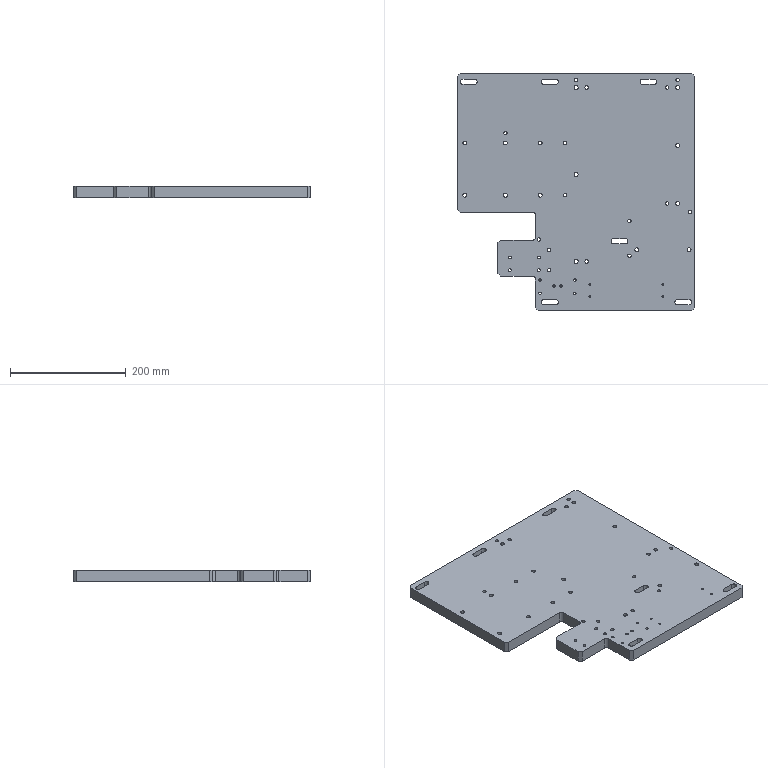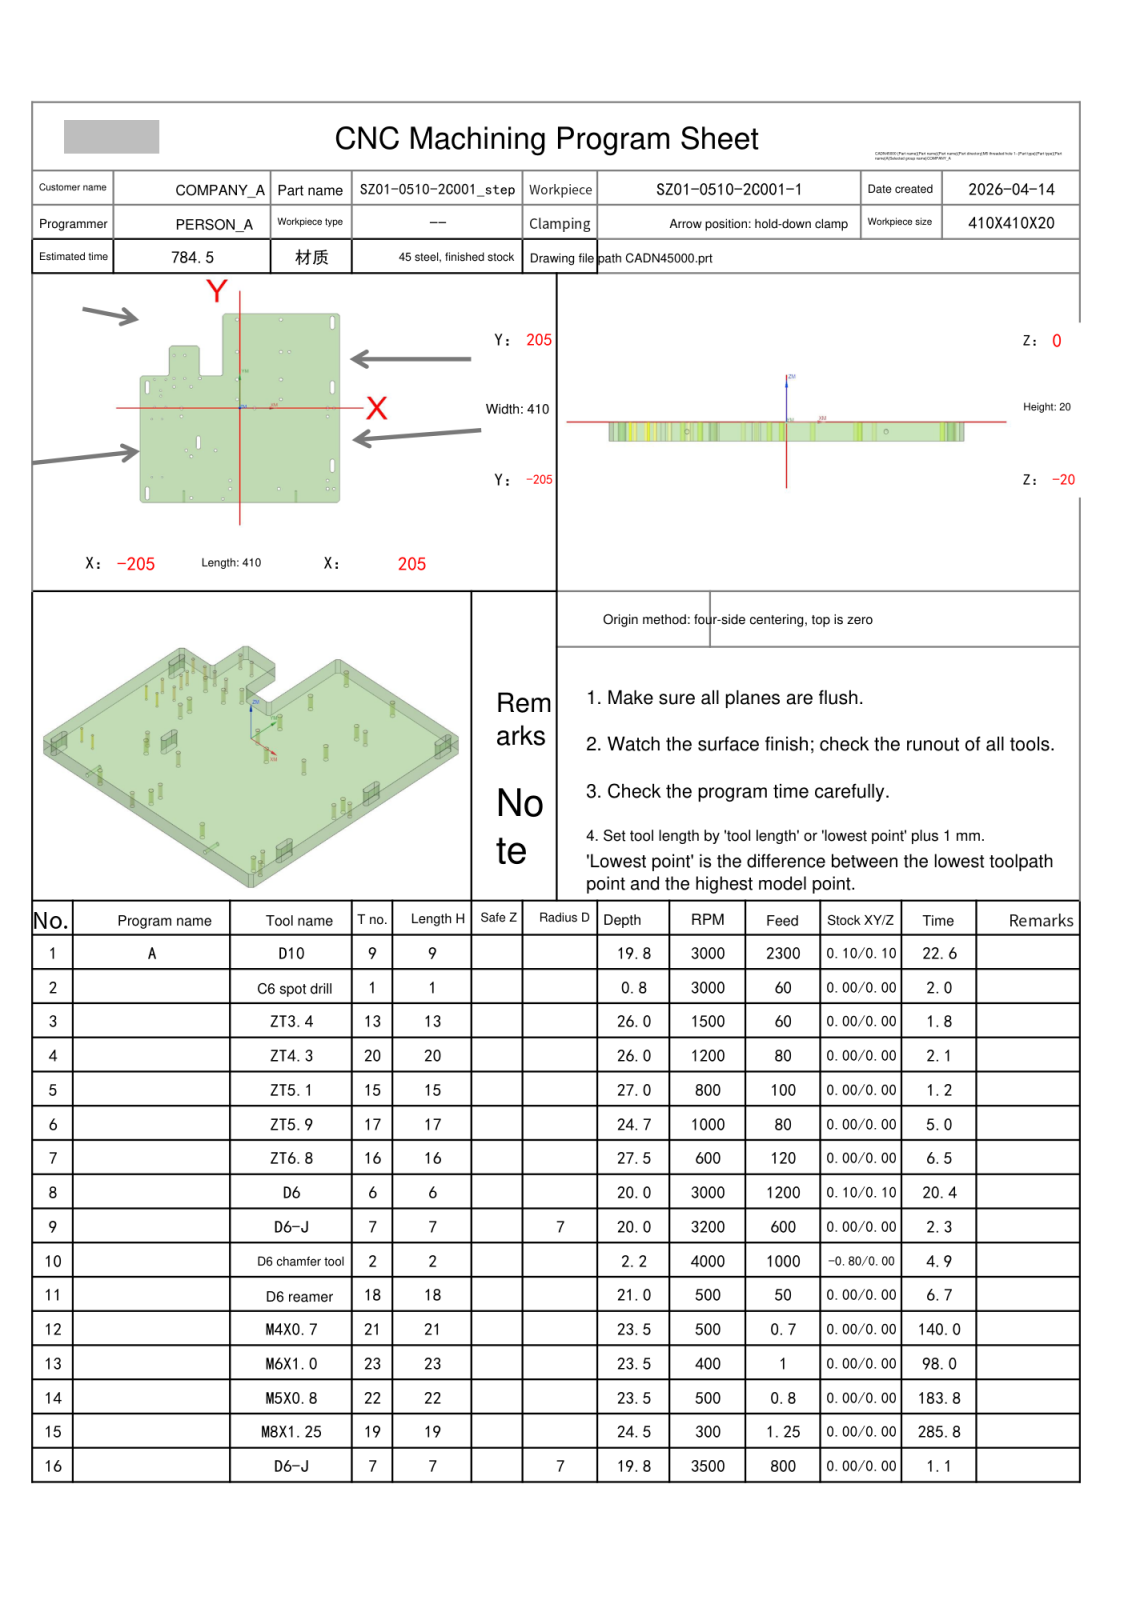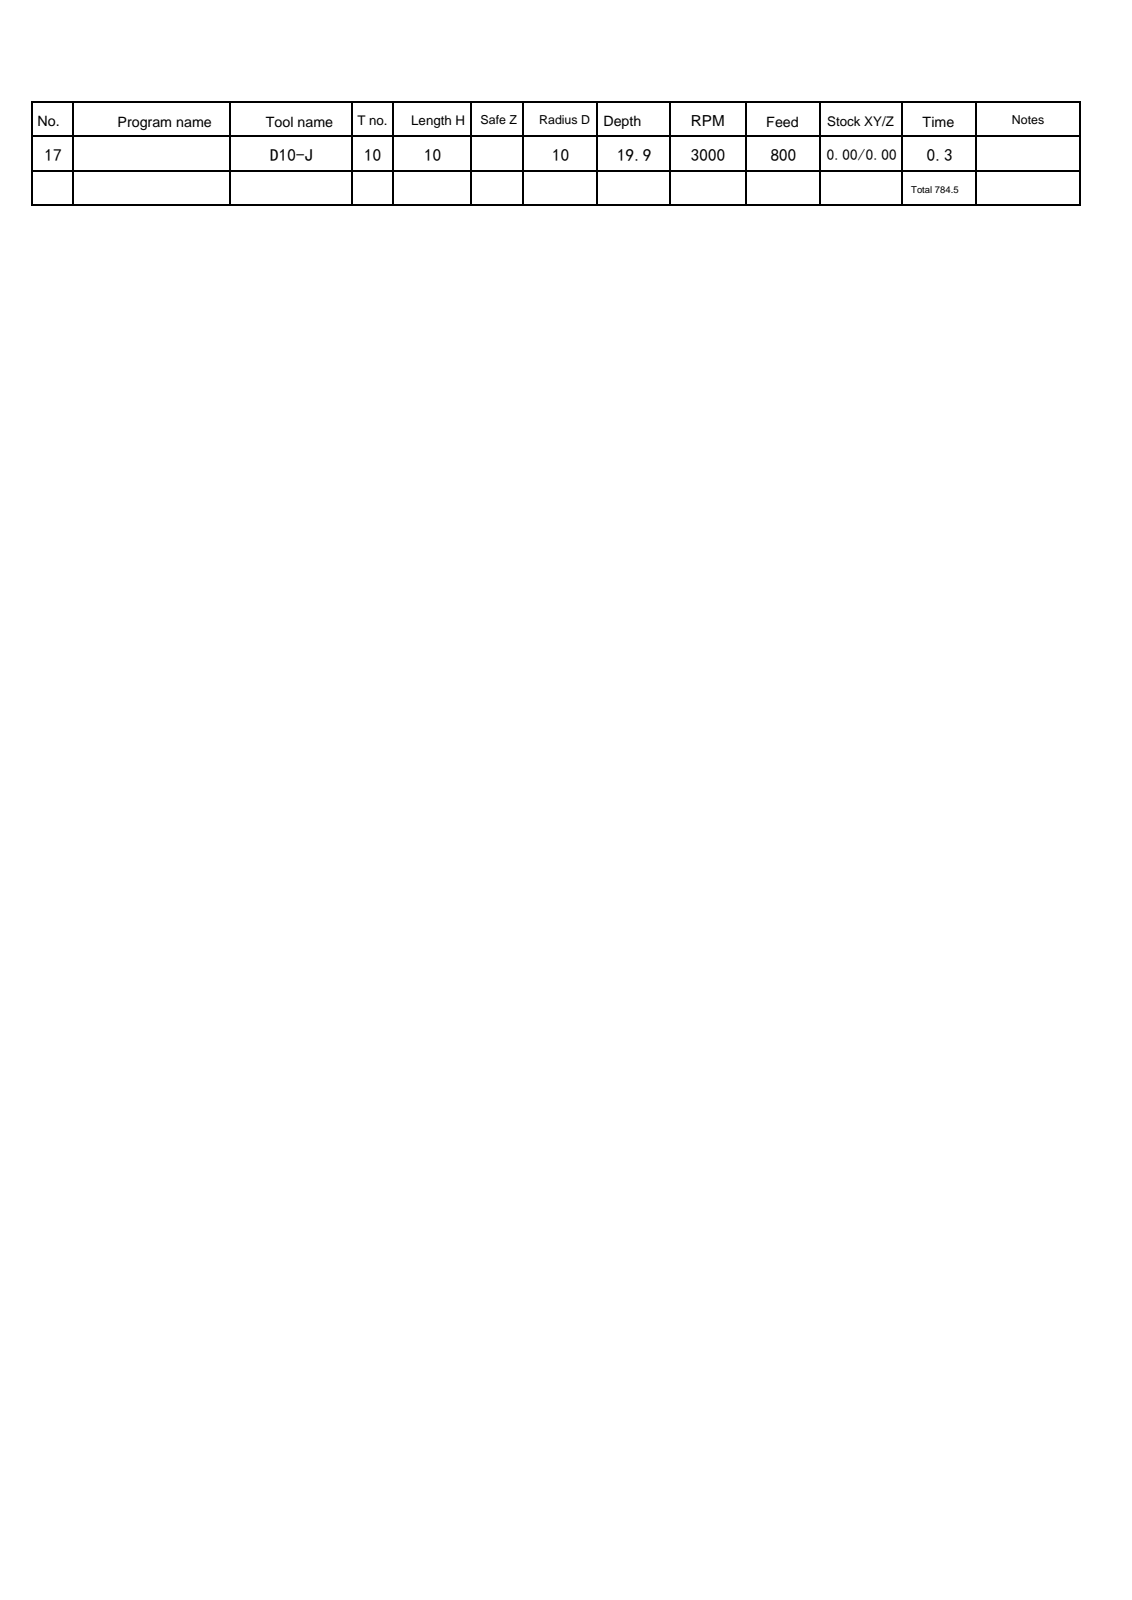NC program | NX | posted by the shop | part box 410 x 410 x 20 mm
Lines 3294 to 4153 of 7905:
N8 T06 M06
(D6  D=6. R=0. H=06 ce=0.10 di=0.10)
G00 G90 G54 X191.4 Y185. M03 S3000
G43 H06 Z50.
M08
Z.5
G01 Y195. Z.449 F1200.
G03 X190. Y196.4 Z.438 I-1.4 J0.0
X188.6 Y195. Z.426 I0.0 J-1.4
G01 Y175. Z.324
G03 X190. Y173.6 Z.313 I1.4 J0.0
X191.4 Y175. Z.301 I0.0 J1.4
G01 Y195. Z.199
G03 X190. Y196.4 Z.188 I-1.4 J0.0
X188.6 Y195. Z.176 I0.0 J-1.4
G01 Y175. Z.074
G03 X190. Y173.6 Z.063 I1.4 J0.0
X191.4 Y175. Z.051 I0.0 J1.4
G01 Y195. Z-.051
G03 X190. Y196.4 Z-.063 I-1.4 J0.0
X188.6 Y195. Z-.074 I0.0 J-1.4
G01 Y175. Z-.176
G03 X190. Y173.6 Z-.188 I1.4 J0.0
X191.4 Y175. Z-.199 I0.0 J1.4
G01 Y195. Z-.301
G03 X190. Y196.4 Z-.313 I-1.4 J0.0
X188.6 Y195. Z-.324 I0.0 J-1.4
G01 Y175. Z-.426
G03 X190. Y173.6 Z-.438 I1.4 J0.0
X191.4 Y175. Z-.449 I0.0 J1.4
G01 Y195. Z-.551
G03 X190. Y196.4 Z-.563 I-1.4 J0.0
X188.6 Y195. Z-.574 I0.0 J-1.4
G01 Y175. Z-.676
G03 X190. Y173.6 Z-.688 I1.4 J0.0
X191.4 Y175. Z-.699 I0.0 J1.4
G01 Y195. Z-.801
G03 X190. Y196.4 Z-.813 I-1.4 J0.0
X188.6 Y195. Z-.824 I0.0 J-1.4
G01 Y175. Z-.926
G03 X190. Y173.6 Z-.938 I1.4 J0.0
X191.4 Y175. Z-.949 I0.0 J1.4
G01 Y195. Z-1.051
G03 X190. Y196.4 Z-1.063 I-1.4 J0.0
X188.6 Y195. Z-1.074 I0.0 J-1.4
G01 Y175. Z-1.176
G03 X190. Y173.6 Z-1.188 I1.4 J0.0
X191.4 Y175. Z-1.199 I0.0 J1.4
G01 Y195. Z-1.301
G03 X190. Y196.4 Z-1.313 I-1.4 J0.0
X188.6 Y195. Z-1.324 I0.0 J-1.4
G01 Y175. Z-1.426
G03 X190. Y173.6 Z-1.438 I1.4 J0.0
X191.4 Y175. Z-1.449 I0.0 J1.4
G01 Y195. Z-1.551
G03 X190. Y196.4 Z-1.563 I-1.4 J0.0
X188.6 Y195. Z-1.574 I0.0 J-1.4
G01 Y175. Z-1.676
G03 X190. Y173.6 Z-1.688 I1.4 J0.0
X191.4 Y175. Z-1.699 I0.0 J1.4
G01 Y195. Z-1.801
G03 X190. Y196.4 Z-1.813 I-1.4 J0.0
X188.6 Y195. Z-1.824 I0.0 J-1.4
G01 Y175. Z-1.926
G03 X190. Y173.6 Z-1.938 I1.4 J0.0
X191.4 Y175. Z-1.949 I0.0 J1.4
G01 Y195. Z-2.051
G03 X190. Y196.4 Z-2.063 I-1.4 J0.0
X188.6 Y195. Z-2.074 I0.0 J-1.4
G01 Y175. Z-2.176
G03 X190. Y173.6 Z-2.188 I1.4 J0.0
X191.4 Y175. Z-2.199 I0.0 J1.4
G01 Y195. Z-2.301
G03 X190. Y196.4 Z-2.313 I-1.4 J0.0
X188.6 Y195. Z-2.324 I0.0 J-1.4
G01 Y175. Z-2.426
G03 X190. Y173.6 Z-2.438 I1.4 J0.0
X191.4 Y175. Z-2.449 I0.0 J1.4
G01 Y195. Z-2.551
G03 X190. Y196.4 Z-2.563 I-1.4 J0.0
X188.6 Y195. Z-2.574 I0.0 J-1.4
G01 Y175. Z-2.676
G03 X190. Y173.6 Z-2.688 I1.4 J0.0
X191.4 Y175. Z-2.699 I0.0 J1.4
G01 Y195. Z-2.801
G03 X190. Y196.4 Z-2.813 I-1.4 J0.0
X188.6 Y195. Z-2.824 I0.0 J-1.4
G01 Y175. Z-2.926
G03 X190. Y173.6 Z-2.938 I1.4 J0.0
X191.4 Y175. Z-2.949 I0.0 J1.4
G01 Y195. Z-3.051
G03 X190. Y196.4 Z-3.063 I-1.4 J0.0
X188.6 Y195. Z-3.074 I0.0 J-1.4
G01 Y175. Z-3.176
G03 X190. Y173.6 Z-3.188 I1.4 J0.0
X191.4 Y175. Z-3.199 I0.0 J1.4
G01 Y195. Z-3.301
G03 X190. Y196.4 Z-3.313 I-1.4 J0.0
X188.6 Y195. Z-3.324 I0.0 J-1.4
G01 Y175. Z-3.426
G03 X190. Y173.6 Z-3.438 I1.4 J0.0
X191.4 Y175. Z-3.449 I0.0 J1.4
G01 Y195. Z-3.551
G03 X190. Y196.4 Z-3.563 I-1.4 J0.0
X188.6 Y195. Z-3.574 I0.0 J-1.4
G01 Y175. Z-3.676
G03 X190. Y173.6 Z-3.688 I1.4 J0.0
X191.4 Y175. Z-3.699 I0.0 J1.4
G01 Y195. Z-3.801
G03 X190. Y196.4 Z-3.813 I-1.4 J0.0
X188.6 Y195. Z-3.824 I0.0 J-1.4
G01 Y175. Z-3.926
G03 X190. Y173.6 Z-3.938 I1.4 J0.0
X191.4 Y175. Z-3.949 I0.0 J1.4
G01 Y195. Z-4.051
G03 X190. Y196.4 Z-4.063 I-1.4 J0.0
X188.6 Y195. Z-4.074 I0.0 J-1.4
G01 Y175. Z-4.176
G03 X190. Y173.6 Z-4.188 I1.4 J0.0
X191.4 Y175. Z-4.199 I0.0 J1.4
G01 Y195. Z-4.301
G03 X190. Y196.4 Z-4.313 I-1.4 J0.0
X188.6 Y195. Z-4.324 I0.0 J-1.4
G01 Y175. Z-4.426
G03 X190. Y173.6 Z-4.438 I1.4 J0.0
X191.4 Y175. Z-4.449 I0.0 J1.4
G01 Y195. Z-4.551
G03 X190. Y196.4 Z-4.563 I-1.4 J0.0
X188.6 Y195. Z-4.574 I0.0 J-1.4
G01 Y175. Z-4.676
G03 X190. Y173.6 Z-4.688 I1.4 J0.0
X191.4 Y175. Z-4.699 I0.0 J1.4
G01 Y195. Z-4.801
G03 X190. Y196.4 Z-4.813 I-1.4 J0.0
X188.6 Y195. Z-4.824 I0.0 J-1.4
G01 Y175. Z-4.926
G03 X190. Y173.6 Z-4.938 I1.4 J0.0
X191.4 Y175. Z-4.949 I0.0 J1.4
G01 Y195. Z-5.051
G03 X190. Y196.4 Z-5.063 I-1.4 J0.0
X188.6 Y195. Z-5.074 I0.0 J-1.4
G01 Y175. Z-5.176
G03 X190. Y173.6 Z-5.188 I1.4 J0.0
X191.4 Y175. Z-5.199 I0.0 J1.4
G01 Y195. Z-5.301
G03 X190. Y196.4 Z-5.313 I-1.4 J0.0
X188.6 Y195. Z-5.324 I0.0 J-1.4
G01 Y175. Z-5.426
G03 X190. Y173.6 Z-5.438 I1.4 J0.0
X191.4 Y175. Z-5.449 I0.0 J1.4
G01 Y195. Z-5.551
G03 X190. Y196.4 Z-5.563 I-1.4 J0.0
X188.6 Y195. Z-5.574 I0.0 J-1.4
G01 Y175. Z-5.676
G03 X190. Y173.6 Z-5.688 I1.4 J0.0
X191.4 Y175. Z-5.699 I0.0 J1.4
G01 Y195. Z-5.801
G03 X190. Y196.4 Z-5.813 I-1.4 J0.0
X188.6 Y195. Z-5.824 I0.0 J-1.4
G01 Y175. Z-5.926
G03 X190. Y173.6 Z-5.938 I1.4 J0.0
X191.4 Y175. Z-5.949 I0.0 J1.4
G01 Y195. Z-6.051
G03 X190. Y196.4 Z-6.063 I-1.4 J0.0
X188.6 Y195. Z-6.074 I0.0 J-1.4
G01 Y175. Z-6.176
G03 X190. Y173.6 Z-6.188 I1.4 J0.0
X191.4 Y175. Z-6.199 I0.0 J1.4
G01 Y195. Z-6.301
G03 X190. Y196.4 Z-6.313 I-1.4 J0.0
X188.6 Y195. Z-6.324 I0.0 J-1.4
G01 Y175. Z-6.426
G03 X190. Y173.6 Z-6.438 I1.4 J0.0
X191.4 Y175. Z-6.449 I0.0 J1.4
G01 Y195. Z-6.551
G03 X190. Y196.4 Z-6.563 I-1.4 J0.0
X188.6 Y195. Z-6.574 I0.0 J-1.4
G01 Y175. Z-6.676
G03 X190. Y173.6 Z-6.688 I1.4 J0.0
X191.4 Y175. Z-6.699 I0.0 J1.4
G01 Y195. Z-6.801
G03 X190. Y196.4 Z-6.813 I-1.4 J0.0
X188.6 Y195. Z-6.824 I0.0 J-1.4
G01 Y175. Z-6.926
G03 X190. Y173.6 Z-6.938 I1.4 J0.0
X191.4 Y175. Z-6.949 I0.0 J1.4
G01 Y195. Z-7.051
G03 X190. Y196.4 Z-7.063 I-1.4 J0.0
X188.6 Y195. Z-7.074 I0.0 J-1.4
G01 Y175. Z-7.176
G03 X190. Y173.6 Z-7.188 I1.4 J0.0
X191.4 Y175. Z-7.199 I0.0 J1.4
G01 Y195. Z-7.301
G03 X190. Y196.4 Z-7.313 I-1.4 J0.0
X188.6 Y195. Z-7.324 I0.0 J-1.4
G01 Y175. Z-7.426
G03 X190. Y173.6 Z-7.438 I1.4 J0.0
X191.4 Y175. Z-7.449 I0.0 J1.4
G01 Y195. Z-7.551
G03 X190. Y196.4 Z-7.563 I-1.4 J0.0
X188.6 Y195. Z-7.574 I0.0 J-1.4
G01 Y175. Z-7.676
G03 X190. Y173.6 Z-7.688 I1.4 J0.0
X191.4 Y175. Z-7.699 I0.0 J1.4
G01 Y195. Z-7.801
G03 X190. Y196.4 Z-7.813 I-1.4 J0.0
X188.6 Y195. Z-7.824 I0.0 J-1.4
G01 Y175. Z-7.926
G03 X190. Y173.6 Z-7.938 I1.4 J0.0
X191.4 Y175. Z-7.949 I0.0 J1.4
G01 Y195. Z-8.051
G03 X190. Y196.4 Z-8.063 I-1.4 J0.0
X188.6 Y195. Z-8.074 I0.0 J-1.4
G01 Y175. Z-8.176
G03 X190. Y173.6 Z-8.188 I1.4 J0.0
X191.4 Y175. Z-8.199 I0.0 J1.4
G01 Y195. Z-8.301
G03 X190. Y196.4 Z-8.313 I-1.4 J0.0
X188.6 Y195. Z-8.324 I0.0 J-1.4
G01 Y175. Z-8.426
G03 X190. Y173.6 Z-8.438 I1.4 J0.0
X191.4 Y175. Z-8.449 I0.0 J1.4
G01 Y195. Z-8.551
G03 X190. Y196.4 Z-8.563 I-1.4 J0.0
X188.6 Y195. Z-8.574 I0.0 J-1.4
G01 Y175. Z-8.676
G03 X190. Y173.6 Z-8.688 I1.4 J0.0
X191.4 Y175. Z-8.699 I0.0 J1.4
G01 Y195. Z-8.801
G03 X190. Y196.4 Z-8.813 I-1.4 J0.0
X188.6 Y195. Z-8.824 I0.0 J-1.4
G01 Y175. Z-8.926
G03 X190. Y173.6 Z-8.938 I1.4 J0.0
X191.4 Y175. Z-8.949 I0.0 J1.4
G01 Y195. Z-9.051
G03 X190. Y196.4 Z-9.063 I-1.4 J0.0
X188.6 Y195. Z-9.074 I0.0 J-1.4
G01 Y175. Z-9.176
G03 X190. Y173.6 Z-9.188 I1.4 J0.0
X191.4 Y175. Z-9.199 I0.0 J1.4
G01 Y195. Z-9.301
G03 X190. Y196.4 Z-9.313 I-1.4 J0.0
X188.6 Y195. Z-9.324 I0.0 J-1.4
G01 Y175. Z-9.426
G03 X190. Y173.6 Z-9.438 I1.4 J0.0
X191.4 Y175. Z-9.449 I0.0 J1.4
G01 Y195. Z-9.551
G03 X190. Y196.4 Z-9.563 I-1.4 J0.0
X188.6 Y195. Z-9.574 I0.0 J-1.4
G01 Y175. Z-9.676
G03 X190. Y173.6 Z-9.688 I1.4 J0.0
X191.4 Y175. Z-9.699 I0.0 J1.4
G01 Y195. Z-9.801
G03 X190. Y196.4 Z-9.813 I-1.4 J0.0
X188.6 Y195. Z-9.824 I0.0 J-1.4
G01 Y175. Z-9.926
G03 X190. Y173.6 Z-9.938 I1.4 J0.0
X191.4 Y175. Z-9.949 I0.0 J1.4
G01 Y195. Z-10.051
G03 X190. Y196.4 Z-10.063 I-1.4 J0.0
X188.6 Y195. Z-10.074 I0.0 J-1.4
G01 Y175. Z-10.176
G03 X190. Y173.6 Z-10.188 I1.4 J0.0
X191.4 Y175. Z-10.199 I0.0 J1.4
G01 Y195. Z-10.301
G03 X190. Y196.4 Z-10.313 I-1.4 J0.0
X188.6 Y195. Z-10.324 I0.0 J-1.4
G01 Y175. Z-10.426
G03 X190. Y173.6 Z-10.438 I1.4 J0.0
X191.4 Y175. Z-10.449 I0.0 J1.4
G01 Y195. Z-10.551
G03 X190. Y196.4 Z-10.563 I-1.4 J0.0
X188.6 Y195. Z-10.574 I0.0 J-1.4
G01 Y175. Z-10.676
G03 X190. Y173.6 Z-10.688 I1.4 J0.0
X191.4 Y175. Z-10.699 I0.0 J1.4
G01 Y195. Z-10.801
G03 X190. Y196.4 Z-10.813 I-1.4 J0.0
X188.6 Y195. Z-10.824 I0.0 J-1.4
G01 Y175. Z-10.926
G03 X190. Y173.6 Z-10.938 I1.4 J0.0
X191.4 Y175. Z-10.949 I0.0 J1.4
G01 Y195. Z-11.051
G03 X190. Y196.4 Z-11.063 I-1.4 J0.0
X188.6 Y195. Z-11.074 I0.0 J-1.4
G01 Y175. Z-11.176
G03 X190. Y173.6 Z-11.188 I1.4 J0.0
X191.4 Y175. Z-11.199 I0.0 J1.4
G01 Y195. Z-11.301
G03 X190. Y196.4 Z-11.313 I-1.4 J0.0
X188.6 Y195. Z-11.324 I0.0 J-1.4
G01 Y175. Z-11.426
G03 X190. Y173.6 Z-11.438 I1.4 J0.0
X191.4 Y175. Z-11.449 I0.0 J1.4
G01 Y195. Z-11.551
G03 X190. Y196.4 Z-11.563 I-1.4 J0.0
X188.6 Y195. Z-11.574 I0.0 J-1.4
G01 Y175. Z-11.676
G03 X190. Y173.6 Z-11.688 I1.4 J0.0
X191.4 Y175. Z-11.699 I0.0 J1.4
G01 Y195. Z-11.801
G03 X190. Y196.4 Z-11.813 I-1.4 J0.0
X188.6 Y195. Z-11.824 I0.0 J-1.4
G01 Y175. Z-11.926
G03 X190. Y173.6 Z-11.938 I1.4 J0.0
X191.4 Y175. Z-11.949 I0.0 J1.4
G01 Y195. Z-12.051
G03 X190. Y196.4 Z-12.063 I-1.4 J0.0
X188.6 Y195. Z-12.074 I0.0 J-1.4
G01 Y175. Z-12.176
G03 X190. Y173.6 Z-12.188 I1.4 J0.0
X191.4 Y175. Z-12.199 I0.0 J1.4
G01 Y195. Z-12.301
G03 X190. Y196.4 Z-12.313 I-1.4 J0.0
X188.6 Y195. Z-12.324 I0.0 J-1.4
G01 Y175. Z-12.426
G03 X190. Y173.6 Z-12.438 I1.4 J0.0
X191.4 Y175. Z-12.449 I0.0 J1.4
G01 Y195. Z-12.551
G03 X190. Y196.4 Z-12.563 I-1.4 J0.0
X188.6 Y195. Z-12.574 I0.0 J-1.4
G01 Y175. Z-12.676
G03 X190. Y173.6 Z-12.688 I1.4 J0.0
X191.4 Y175. Z-12.699 I0.0 J1.4
G01 Y195. Z-12.801
G03 X190. Y196.4 Z-12.813 I-1.4 J0.0
X188.6 Y195. Z-12.824 I0.0 J-1.4
G01 Y175. Z-12.926
G03 X190. Y173.6 Z-12.938 I1.4 J0.0
X191.4 Y175. Z-12.949 I0.0 J1.4
G01 Y195. Z-13.051
G03 X190. Y196.4 Z-13.063 I-1.4 J0.0
X188.6 Y195. Z-13.074 I0.0 J-1.4
G01 Y175. Z-13.176
G03 X190. Y173.6 Z-13.188 I1.4 J0.0
X191.4 Y175. Z-13.199 I0.0 J1.4
G01 Y195. Z-13.301
G03 X190. Y196.4 Z-13.313 I-1.4 J0.0
X188.6 Y195. Z-13.324 I0.0 J-1.4
G01 Y175. Z-13.426
G03 X190. Y173.6 Z-13.438 I1.4 J0.0
X191.4 Y175. Z-13.449 I0.0 J1.4
G01 Y195. Z-13.551
G03 X190. Y196.4 Z-13.563 I-1.4 J0.0
X188.6 Y195. Z-13.574 I0.0 J-1.4
G01 Y175. Z-13.676
G03 X190. Y173.6 Z-13.688 I1.4 J0.0
X191.4 Y175. Z-13.699 I0.0 J1.4
G01 Y195. Z-13.801
G03 X190. Y196.4 Z-13.813 I-1.4 J0.0
X188.6 Y195. Z-13.824 I0.0 J-1.4
G01 Y175. Z-13.926
G03 X190. Y173.6 Z-13.938 I1.4 J0.0
X191.4 Y175. Z-13.949 I0.0 J1.4
G01 Y195. Z-14.051
G03 X190. Y196.4 Z-14.063 I-1.4 J0.0
X188.6 Y195. Z-14.074 I0.0 J-1.4
G01 Y175. Z-14.176
G03 X190. Y173.6 Z-14.188 I1.4 J0.0
X191.4 Y175. Z-14.199 I0.0 J1.4
G01 Y195. Z-14.301
G03 X190. Y196.4 Z-14.313 I-1.4 J0.0
X188.6 Y195. Z-14.324 I0.0 J-1.4
G01 Y175. Z-14.426
G03 X190. Y173.6 Z-14.438 I1.4 J0.0
X191.4 Y175. Z-14.449 I0.0 J1.4
G01 Y195. Z-14.551
G03 X190. Y196.4 Z-14.563 I-1.4 J0.0
X188.6 Y195. Z-14.574 I0.0 J-1.4
G01 Y175. Z-14.676
G03 X190. Y173.6 Z-14.688 I1.4 J0.0
X191.4 Y175. Z-14.699 I0.0 J1.4
G01 Y195. Z-14.801
G03 X190. Y196.4 Z-14.813 I-1.4 J0.0
X188.6 Y195. Z-14.824 I0.0 J-1.4
G01 Y175. Z-14.926
G03 X190. Y173.6 Z-14.938 I1.4 J0.0
X191.4 Y175. Z-14.949 I0.0 J1.4
G01 Y195. Z-15.051
G03 X190. Y196.4 Z-15.063 I-1.4 J0.0
X188.6 Y195. Z-15.074 I0.0 J-1.4
G01 Y175. Z-15.176
G03 X190. Y173.6 Z-15.188 I1.4 J0.0
X191.4 Y175. Z-15.199 I0.0 J1.4
G01 Y195. Z-15.301
G03 X190. Y196.4 Z-15.313 I-1.4 J0.0
X188.6 Y195. Z-15.324 I0.0 J-1.4
G01 Y175. Z-15.426
G03 X190. Y173.6 Z-15.438 I1.4 J0.0
X191.4 Y175. Z-15.449 I0.0 J1.4
G01 Y195. Z-15.551
G03 X190. Y196.4 Z-15.563 I-1.4 J0.0
X188.6 Y195. Z-15.574 I0.0 J-1.4
G01 Y175. Z-15.676
G03 X190. Y173.6 Z-15.688 I1.4 J0.0
X191.4 Y175. Z-15.699 I0.0 J1.4
G01 Y195. Z-15.801
G03 X190. Y196.4 Z-15.813 I-1.4 J0.0
X188.6 Y195. Z-15.824 I0.0 J-1.4
G01 Y175. Z-15.926
G03 X190. Y173.6 Z-15.938 I1.4 J0.0
X191.4 Y175. Z-15.949 I0.0 J1.4
G01 Y195. Z-16.051
G03 X190. Y196.4 Z-16.063 I-1.4 J0.0
X188.6 Y195. Z-16.074 I0.0 J-1.4
G01 Y175. Z-16.176
G03 X190. Y173.6 Z-16.188 I1.4 J0.0
X191.4 Y175. Z-16.199 I0.0 J1.4
G01 Y195. Z-16.301
G03 X190. Y196.4 Z-16.313 I-1.4 J0.0
X188.6 Y195. Z-16.324 I0.0 J-1.4
G01 Y175. Z-16.426
G03 X190. Y173.6 Z-16.438 I1.4 J0.0
X191.4 Y175. Z-16.449 I0.0 J1.4
G01 Y195. Z-16.551
G03 X190. Y196.4 Z-16.563 I-1.4 J0.0
X188.6 Y195. Z-16.574 I0.0 J-1.4
G01 Y175. Z-16.676
G03 X190. Y173.6 Z-16.688 I1.4 J0.0
X191.4 Y175. Z-16.699 I0.0 J1.4
G01 Y195. Z-16.801
G03 X190. Y196.4 Z-16.813 I-1.4 J0.0
X188.6 Y195. Z-16.824 I0.0 J-1.4
G01 Y175. Z-16.926
G03 X190. Y173.6 Z-16.938 I1.4 J0.0
X191.4 Y175. Z-16.949 I0.0 J1.4
G01 Y195. Z-17.051
G03 X190. Y196.4 Z-17.063 I-1.4 J0.0
X188.6 Y195. Z-17.074 I0.0 J-1.4
G01 Y175. Z-17.176
G03 X190. Y173.6 Z-17.188 I1.4 J0.0
X191.4 Y175. Z-17.199 I0.0 J1.4
G01 Y195. Z-17.301
G03 X190. Y196.4 Z-17.313 I-1.4 J0.0
X188.6 Y195. Z-17.324 I0.0 J-1.4
G01 Y175. Z-17.426
G03 X190. Y173.6 Z-17.438 I1.4 J0.0
X191.4 Y175. Z-17.449 I0.0 J1.4
G01 Y195. Z-17.551
G03 X190. Y196.4 Z-17.563 I-1.4 J0.0
X188.6 Y195. Z-17.574 I0.0 J-1.4
G01 Y175. Z-17.676
G03 X190. Y173.6 Z-17.688 I1.4 J0.0
X191.4 Y175. Z-17.699 I0.0 J1.4
G01 Y195. Z-17.801
G03 X190. Y196.4 Z-17.813 I-1.4 J0.0
X188.6 Y195. Z-17.824 I0.0 J-1.4
G01 Y175. Z-17.926
G03 X190. Y173.6 Z-17.938 I1.4 J0.0
X191.4 Y175. Z-17.949 I0.0 J1.4
G01 Y195. Z-18.051
G03 X190. Y196.4 Z-18.063 I-1.4 J0.0
X188.6 Y195. Z-18.074 I0.0 J-1.4
G01 Y175. Z-18.176
G03 X190. Y173.6 Z-18.188 I1.4 J0.0
X191.4 Y175. Z-18.199 I0.0 J1.4
G01 Y195. Z-18.301
G03 X190. Y196.4 Z-18.313 I-1.4 J0.0
X188.6 Y195. Z-18.324 I0.0 J-1.4
G01 Y175. Z-18.426
G03 X190. Y173.6 Z-18.438 I1.4 J0.0
X191.4 Y175. Z-18.449 I0.0 J1.4
G01 Y195. Z-18.551
G03 X190. Y196.4 Z-18.563 I-1.4 J0.0
X188.6 Y195. Z-18.574 I0.0 J-1.4
G01 Y175. Z-18.676
G03 X190. Y173.6 Z-18.688 I1.4 J0.0
X191.4 Y175. Z-18.699 I0.0 J1.4
G01 Y195. Z-18.801
G03 X190. Y196.4 Z-18.813 I-1.4 J0.0
X188.6 Y195. Z-18.824 I0.0 J-1.4
G01 Y175. Z-18.926
G03 X190. Y173.6 Z-18.938 I1.4 J0.0
X191.4 Y175. Z-18.949 I0.0 J1.4
G01 Y195. Z-19.051
G03 X190. Y196.4 Z-19.063 I-1.4 J0.0
X188.6 Y195. Z-19.074 I0.0 J-1.4
G01 Y175. Z-19.176
G03 X190. Y173.6 Z-19.188 I1.4 J0.0
X191.4 Y175. Z-19.199 I0.0 J1.4
G01 Y195. Z-19.301
G03 X190. Y196.4 Z-19.313 I-1.4 J0.0
X188.6 Y195. Z-19.324 I0.0 J-1.4
G01 Y175. Z-19.426
G03 X190. Y173.6 Z-19.438 I1.4 J0.0
X191.4 Y175. Z-19.449 I0.0 J1.4
G01 Y195. Z-19.551
G03 X190. Y196.4 Z-19.563 I-1.4 J0.0
X188.6 Y195. Z-19.574 I0.0 J-1.4
G01 Y175. Z-19.676
G03 X190. Y173.6 Z-19.688 I1.4 J0.0
X191.4 Y175. Z-19.699 I0.0 J1.4
G01 Y195. Z-19.801
G03 X190. Y196.4 Z-19.813 I-1.4 J0.0
X188.6 Y195. Z-19.824 I0.0 J-1.4
G01 Y175. Z-19.926
G03 X190. Y173.6 Z-19.938 I1.4 J0.0
X191.4 Y175. Z-19.949 I0.0 J1.4
G01 Y185. Z-20.
Y195.
G03 X190. Y196.4 I-1.4 J0.0
X188.6 Y195. I0.0 J-1.4
G01 Y175.
G03 X190. Y173.6 I1.4 J0.0
X191.4 Y175. I0.0 J1.4
G01 Y185.
Y185.5
Z-19.
G00 Z50.
Y45.
Z.5
G01 Y55. Z.449
G03 X190. Y56.4 Z.438 I-1.4 J0.0
X188.6 Y55. Z.426 I0.0 J-1.4
G01 Y35. Z.324
G03 X190. Y33.6 Z.313 I1.4 J0.0
X191.4 Y35. Z.301 I0.0 J1.4
G01 Y55. Z.199
G03 X190. Y56.4 Z.188 I-1.4 J0.0
X188.6 Y55. Z.176 I0.0 J-1.4
G01 Y35. Z.074
G03 X190. Y33.6 Z.063 I1.4 J0.0
X191.4 Y35. Z.051 I0.0 J1.4
G01 Y55. Z-.051
G03 X190. Y56.4 Z-.063 I-1.4 J0.0
X188.6 Y55. Z-.074 I0.0 J-1.4
G01 Y35. Z-.176
G03 X190. Y33.6 Z-.188 I1.4 J0.0
X191.4 Y35. Z-.199 I0.0 J1.4
G01 Y55. Z-.301
G03 X190. Y56.4 Z-.313 I-1.4 J0.0
X188.6 Y55. Z-.324 I0.0 J-1.4
G01 Y35. Z-.426
G03 X190. Y33.6 Z-.438 I1.4 J0.0
X191.4 Y35. Z-.449 I0.0 J1.4
G01 Y55. Z-.551
G03 X190. Y56.4 Z-.563 I-1.4 J0.0
X188.6 Y55. Z-.574 I0.0 J-1.4
G01 Y35. Z-.676
G03 X190. Y33.6 Z-.688 I1.4 J0.0
X191.4 Y35. Z-.699 I0.0 J1.4
G01 Y55. Z-.801
G03 X190. Y56.4 Z-.813 I-1.4 J0.0
X188.6 Y55. Z-.824 I0.0 J-1.4
G01 Y35. Z-.926
G03 X190. Y33.6 Z-.938 I1.4 J0.0
X191.4 Y35. Z-.949 I0.0 J1.4
G01 Y55. Z-1.051
G03 X190. Y56.4 Z-1.063 I-1.4 J0.0
X188.6 Y55. Z-1.074 I0.0 J-1.4
G01 Y35. Z-1.176
G03 X190. Y33.6 Z-1.188 I1.4 J0.0
X191.4 Y35. Z-1.199 I0.0 J1.4
G01 Y55. Z-1.301
G03 X190. Y56.4 Z-1.313 I-1.4 J0.0
X188.6 Y55. Z-1.324 I0.0 J-1.4
G01 Y35. Z-1.426
G03 X190. Y33.6 Z-1.438 I1.4 J0.0
X191.4 Y35. Z-1.449 I0.0 J1.4
G01 Y55. Z-1.551
G03 X190. Y56.4 Z-1.563 I-1.4 J0.0
X188.6 Y55. Z-1.574 I0.0 J-1.4
G01 Y35. Z-1.676
G03 X190. Y33.6 Z-1.688 I1.4 J0.0
X191.4 Y35. Z-1.699 I0.0 J1.4
G01 Y55. Z-1.801
G03 X190. Y56.4 Z-1.813 I-1.4 J0.0
X188.6 Y55. Z-1.824 I0.0 J-1.4
G01 Y35. Z-1.926
G03 X190. Y33.6 Z-1.938 I1.4 J0.0
X191.4 Y35. Z-1.949 I0.0 J1.4
G01 Y55. Z-2.051
G03 X190. Y56.4 Z-2.063 I-1.4 J0.0
X188.6 Y55. Z-2.074 I0.0 J-1.4
G01 Y35. Z-2.176
G03 X190. Y33.6 Z-2.188 I1.4 J0.0
X191.4 Y35. Z-2.199 I0.0 J1.4
G01 Y55. Z-2.301
G03 X190. Y56.4 Z-2.313 I-1.4 J0.0
X188.6 Y55. Z-2.324 I0.0 J-1.4
G01 Y35. Z-2.426
G03 X190. Y33.6 Z-2.438 I1.4 J0.0
X191.4 Y35. Z-2.449 I0.0 J1.4
G01 Y55. Z-2.551
G03 X190. Y56.4 Z-2.563 I-1.4 J0.0
X188.6 Y55. Z-2.574 I0.0 J-1.4
G01 Y35. Z-2.676
G03 X190. Y33.6 Z-2.688 I1.4 J0.0
X191.4 Y35. Z-2.699 I0.0 J1.4
G01 Y55. Z-2.801
G03 X190. Y56.4 Z-2.813 I-1.4 J0.0
X188.6 Y55. Z-2.824 I0.0 J-1.4
G01 Y35. Z-2.926
G03 X190. Y33.6 Z-2.938 I1.4 J0.0
X191.4 Y35. Z-2.949 I0.0 J1.4
G01 Y55. Z-3.051
G03 X190. Y56.4 Z-3.063 I-1.4 J0.0
X188.6 Y55. Z-3.074 I0.0 J-1.4
G01 Y35. Z-3.176
G03 X190. Y33.6 Z-3.188 I1.4 J0.0
X191.4 Y35. Z-3.199 I0.0 J1.4
G01 Y55. Z-3.301
G03 X190. Y56.4 Z-3.313 I-1.4 J0.0
X188.6 Y55. Z-3.324 I0.0 J-1.4
G01 Y35. Z-3.426
G03 X190. Y33.6 Z-3.438 I1.4 J0.0
X191.4 Y35. Z-3.449 I0.0 J1.4
G01 Y55. Z-3.551
G03 X190. Y56.4 Z-3.563 I-1.4 J0.0
X188.6 Y55. Z-3.574 I0.0 J-1.4
G01 Y35. Z-3.676
G03 X190. Y33.6 Z-3.688 I1.4 J0.0
X191.4 Y35. Z-3.699 I0.0 J1.4
G01 Y55. Z-3.801
G03 X190. Y56.4 Z-3.813 I-1.4 J0.0
X188.6 Y55. Z-3.824 I0.0 J-1.4
G01 Y35. Z-3.926
G03 X190. Y33.6 Z-3.938 I1.4 J0.0
X191.4 Y35. Z-3.949 I0.0 J1.4
G01 Y55. Z-4.051
G03 X190. Y56.4 Z-4.063 I-1.4 J0.0
X188.6 Y55. Z-4.074 I0.0 J-1.4
G01 Y35. Z-4.176
G03 X190. Y33.6 Z-4.188 I1.4 J0.0
X191.4 Y35. Z-4.199 I0.0 J1.4
G01 Y55. Z-4.301
G03 X190. Y56.4 Z-4.313 I-1.4 J0.0
X188.6 Y55. Z-4.324 I0.0 J-1.4
G01 Y35. Z-4.426
G03 X190. Y33.6 Z-4.438 I1.4 J0.0
X191.4 Y35. Z-4.449 I0.0 J1.4
G01 Y55. Z-4.551
G03 X190. Y56.4 Z-4.563 I-1.4 J0.0
X188.6 Y55. Z-4.574 I0.0 J-1.4
G01 Y35. Z-4.676
G03 X190. Y33.6 Z-4.688 I1.4 J0.0
X191.4 Y35. Z-4.699 I0.0 J1.4
G01 Y55. Z-4.801
G03 X190. Y56.4 Z-4.813 I-1.4 J0.0
X188.6 Y55. Z-4.824 I0.0 J-1.4
G01 Y35. Z-4.926
G03 X190. Y33.6 Z-4.938 I1.4 J0.0
X191.4 Y35. Z-4.949 I0.0 J1.4
G01 Y55. Z-5.051
G03 X190. Y56.4 Z-5.063 I-1.4 J0.0
X188.6 Y55. Z-5.074 I0.0 J-1.4
G01 Y35. Z-5.176
G03 X190. Y33.6 Z-5.188 I1.4 J0.0
X191.4 Y35. Z-5.199 I0.0 J1.4
G01 Y55. Z-5.301
G03 X190. Y56.4 Z-5.313 I-1.4 J0.0
X188.6 Y55. Z-5.324 I0.0 J-1.4
G01 Y35. Z-5.426
G03 X190. Y33.6 Z-5.438 I1.4 J0.0
X191.4 Y35. Z-5.449 I0.0 J1.4
G01 Y55. Z-5.551
G03 X190. Y56.4 Z-5.563 I-1.4 J0.0
X188.6 Y55. Z-5.574 I0.0 J-1.4
G01 Y35. Z-5.676
G03 X190. Y33.6 Z-5.688 I1.4 J0.0
X191.4 Y35. Z-5.699 I0.0 J1.4
G01 Y55. Z-5.801
G03 X190. Y56.4 Z-5.813 I-1.4 J0.0
X188.6 Y55. Z-5.824 I0.0 J-1.4
G01 Y35. Z-5.926
G03 X190. Y33.6 Z-5.938 I1.4 J0.0
X191.4 Y35. Z-5.949 I0.0 J1.4
G01 Y55. Z-6.051
G03 X190. Y56.4 Z-6.063 I-1.4 J0.0
X188.6 Y55. Z-6.074 I0.0 J-1.4
G01 Y35. Z-6.176
G03 X190. Y33.6 Z-6.188 I1.4 J0.0
X191.4 Y35. Z-6.199 I0.0 J1.4
G01 Y55. Z-6.301
G03 X190. Y56.4 Z-6.313 I-1.4 J0.0
X188.6 Y55. Z-6.324 I0.0 J-1.4
G01 Y35. Z-6.426
G03 X190. Y33.6 Z-6.438 I1.4 J0.0
X191.4 Y35. Z-6.449 I0.0 J1.4
G01 Y55. Z-6.551
G03 X190. Y56.4 Z-6.563 I-1.4 J0.0
X188.6 Y55. Z-6.574 I0.0 J-1.4
G01 Y35. Z-6.676
G03 X190. Y33.6 Z-6.688 I1.4 J0.0
X191.4 Y35. Z-6.699 I0.0 J1.4
G01 Y55. Z-6.801
G03 X190. Y56.4 Z-6.813 I-1.4 J0.0
X188.6 Y55. Z-6.824 I0.0 J-1.4
G01 Y35. Z-6.926
G03 X190. Y33.6 Z-6.938 I1.4 J0.0
X191.4 Y35. Z-6.949 I0.0 J1.4
G01 Y55. Z-7.051
G03 X190. Y56.4 Z-7.063 I-1.4 J0.0
X188.6 Y55. Z-7.074 I0.0 J-1.4
G01 Y35. Z-7.176
G03 X190. Y33.6 Z-7.188 I1.4 J0.0
X191.4 Y35. Z-7.199 I0.0 J1.4
G01 Y55. Z-7.301
G03 X190. Y56.4 Z-7.313 I-1.4 J0.0
X188.6 Y55. Z-7.324 I0.0 J-1.4
G01 Y35. Z-7.426
G03 X190. Y33.6 Z-7.438 I1.4 J0.0
X191.4 Y35. Z-7.449 I0.0 J1.4
G01 Y55. Z-7.551
G03 X190. Y56.4 Z-7.563 I-1.4 J0.0
X188.6 Y55. Z-7.574 I0.0 J-1.4
G01 Y35. Z-7.676
G03 X190. Y33.6 Z-7.688 I1.4 J0.0
X191.4 Y35. Z-7.699 I0.0 J1.4
G01 Y55. Z-7.801
G03 X190. Y56.4 Z-7.813 I-1.4 J0.0
X188.6 Y55. Z-7.824 I0.0 J-1.4
G01 Y35. Z-7.926
G03 X190. Y33.6 Z-7.938 I1.4 J0.0
X191.4 Y35. Z-7.949 I0.0 J1.4
G01 Y55. Z-8.051
G03 X190. Y56.4 Z-8.063 I-1.4 J0.0
X188.6 Y55. Z-8.074 I0.0 J-1.4
G01 Y35. Z-8.176
G03 X190. Y33.6 Z-8.188 I1.4 J0.0
X191.4 Y35. Z-8.199 I0.0 J1.4
G01 Y55. Z-8.301
G03 X190. Y56.4 Z-8.313 I-1.4 J0.0
X188.6 Y55. Z-8.324 I0.0 J-1.4
G01 Y35. Z-8.426
G03 X190. Y33.6 Z-8.438 I1.4 J0.0
X191.4 Y35. Z-8.449 I0.0 J1.4
G01 Y55. Z-8.551
G03 X190. Y56.4 Z-8.563 I-1.4 J0.0
X188.6 Y55. Z-8.574 I0.0 J-1.4
G01 Y35. Z-8.676
G03 X190. Y33.6 Z-8.688 I1.4 J0.0
X191.4 Y35. Z-8.699 I0.0 J1.4
G01 Y55. Z-8.801
G03 X190. Y56.4 Z-8.813 I-1.4 J0.0
X188.6 Y55. Z-8.824 I0.0 J-1.4
G01 Y35. Z-8.926
G03 X190. Y33.6 Z-8.938 I1.4 J0.0
X191.4 Y35. Z-8.949 I0.0 J1.4
G01 Y55. Z-9.051
G03 X190. Y56.4 Z-9.063 I-1.4 J0.0
X188.6 Y55. Z-9.074 I0.0 J-1.4
G01 Y35. Z-9.176
G03 X190. Y33.6 Z-9.188 I1.4 J0.0
X191.4 Y35. Z-9.199 I0.0 J1.4
G01 Y55. Z-9.301
G03 X190. Y56.4 Z-9.313 I-1.4 J0.0
X188.6 Y55. Z-9.324 I0.0 J-1.4
G01 Y35. Z-9.426
G03 X190. Y33.6 Z-9.438 I1.4 J0.0
X191.4 Y35. Z-9.449 I0.0 J1.4
G01 Y55. Z-9.551
G03 X190. Y56.4 Z-9.563 I-1.4 J0.0
X188.6 Y55. Z-9.574 I0.0 J-1.4
G01 Y35. Z-9.676
G03 X190. Y33.6 Z-9.688 I1.4 J0.0
X191.4 Y35. Z-9.699 I0.0 J1.4
G01 Y55. Z-9.801
G03 X190. Y56.4 Z-9.813 I-1.4 J0.0
X188.6 Y55. Z-9.824 I0.0 J-1.4
G01 Y35. Z-9.926
G03 X190. Y33.6 Z-9.938 I1.4 J0.0
X191.4 Y35. Z-9.949 I0.0 J1.4
G01 Y55. Z-10.051
G03 X190. Y56.4 Z-10.063 I-1.4 J0.0
X188.6 Y55. Z-10.074 I0.0 J-1.4
G01 Y35. Z-10.176
G03 X190. Y33.6 Z-10.188 I1.4 J0.0
X191.4 Y35. Z-10.199 I0.0 J1.4
G01 Y55. Z-10.301
G03 X190. Y56.4 Z-10.313 I-1.4 J0.0
X188.6 Y55. Z-10.324 I0.0 J-1.4
G01 Y35. Z-10.426
G03 X190. Y33.6 Z-10.438 I1.4 J0.0
X191.4 Y35. Z-10.449 I0.0 J1.4
G01 Y55. Z-10.551
G03 X190. Y56.4 Z-10.563 I-1.4 J0.0
X188.6 Y55. Z-10.574 I0.0 J-1.4
G01 Y35. Z-10.676
G03 X190. Y33.6 Z-10.688 I1.4 J0.0
X191.4 Y35. Z-10.699 I0.0 J1.4
G01 Y55. Z-10.801
G03 X190. Y56.4 Z-10.813 I-1.4 J0.0
X188.6 Y55. Z-10.824 I0.0 J-1.4
G01 Y35. Z-10.926
G03 X190. Y33.6 Z-10.938 I1.4 J0.0
X191.4 Y35. Z-10.949 I0.0 J1.4
G01 Y55. Z-11.051
G03 X190. Y56.4 Z-11.063 I-1.4 J0.0
X188.6 Y55. Z-11.074 I0.0 J-1.4
G01 Y35. Z-11.176
G03 X190. Y33.6 Z-11.188 I1.4 J0.0
X191.4 Y35. Z-11.199 I0.0 J1.4
G01 Y55. Z-11.301
G03 X190. Y56.4 Z-11.313 I-1.4 J0.0
X188.6 Y55. Z-11.324 I0.0 J-1.4
G01 Y35. Z-11.426
G03 X190. Y33.6 Z-11.438 I1.4 J0.0
X191.4 Y35. Z-11.449 I0.0 J1.4
G01 Y55. Z-11.551
G03 X190. Y56.4 Z-11.563 I-1.4 J0.0
X188.6 Y55. Z-11.574 I0.0 J-1.4
G01 Y35. Z-11.676
G03 X190. Y33.6 Z-11.688 I1.4 J0.0
X191.4 Y35. Z-11.699 I0.0 J1.4
G01 Y55. Z-11.801
G03 X190. Y56.4 Z-11.813 I-1.4 J0.0
X188.6 Y55. Z-11.824 I0.0 J-1.4
G01 Y35. Z-11.926
G03 X190. Y33.6 Z-11.938 I1.4 J0.0
X191.4 Y35. Z-11.949 I0.0 J1.4
G01 Y55. Z-12.051
G03 X190. Y56.4 Z-12.063 I-1.4 J0.0
X188.6 Y55. Z-12.074 I0.0 J-1.4
G01 Y35. Z-12.176
G03 X190. Y33.6 Z-12.188 I1.4 J0.0
X191.4 Y35. Z-12.199 I0.0 J1.4
G01 Y55. Z-12.301
G03 X190. Y56.4 Z-12.313 I-1.4 J0.0
X188.6 Y55. Z-12.324 I0.0 J-1.4
G01 Y35. Z-12.426
G03 X190. Y33.6 Z-12.438 I1.4 J0.0
X191.4 Y35. Z-12.449 I0.0 J1.4
G01 Y55. Z-12.551
G03 X190. Y56.4 Z-12.563 I-1.4 J0.0
X188.6 Y55. Z-12.574 I0.0 J-1.4
G01 Y35. Z-12.676
G03 X190. Y33.6 Z-12.688 I1.4 J0.0
X191.4 Y35. Z-12.699 I0.0 J1.4
G01 Y55. Z-12.801
G03 X190. Y56.4 Z-12.813 I-1.4 J0.0
X188.6 Y55. Z-12.824 I0.0 J-1.4
G01 Y35. Z-12.926
G03 X190. Y33.6 Z-12.938 I1.4 J0.0
X191.4 Y35. Z-12.949 I0.0 J1.4
G01 Y55. Z-13.051
G03 X190. Y56.4 Z-13.063 I-1.4 J0.0
X188.6 Y55. Z-13.074 I0.0 J-1.4
G01 Y35. Z-13.176
G03 X190. Y33.6 Z-13.188 I1.4 J0.0
X191.4 Y35. Z-13.199 I0.0 J1.4
G01 Y55. Z-13.301
G03 X190. Y56.4 Z-13.313 I-1.4 J0.0
X188.6 Y55. Z-13.324 I0.0 J-1.4
G01 Y35. Z-13.426
G03 X190. Y33.6 Z-13.438 I1.4 J0.0
X191.4 Y35. Z-13.449 I0.0 J1.4
G01 Y55. Z-13.551
G03 X190. Y56.4 Z-13.563 I-1.4 J0.0
X188.6 Y55. Z-13.574 I0.0 J-1.4
G01 Y35. Z-13.676
G03 X190. Y33.6 Z-13.688 I1.4 J0.0
X191.4 Y35. Z-13.699 I0.0 J1.4
G01 Y55. Z-13.801
G03 X190. Y56.4 Z-13.813 I-1.4 J0.0
X188.6 Y55. Z-13.824 I0.0 J-1.4
G01 Y35. Z-13.926
G03 X190. Y33.6 Z-13.938 I1.4 J0.0
X191.4 Y35. Z-13.949 I0.0 J1.4
G01 Y55. Z-14.051